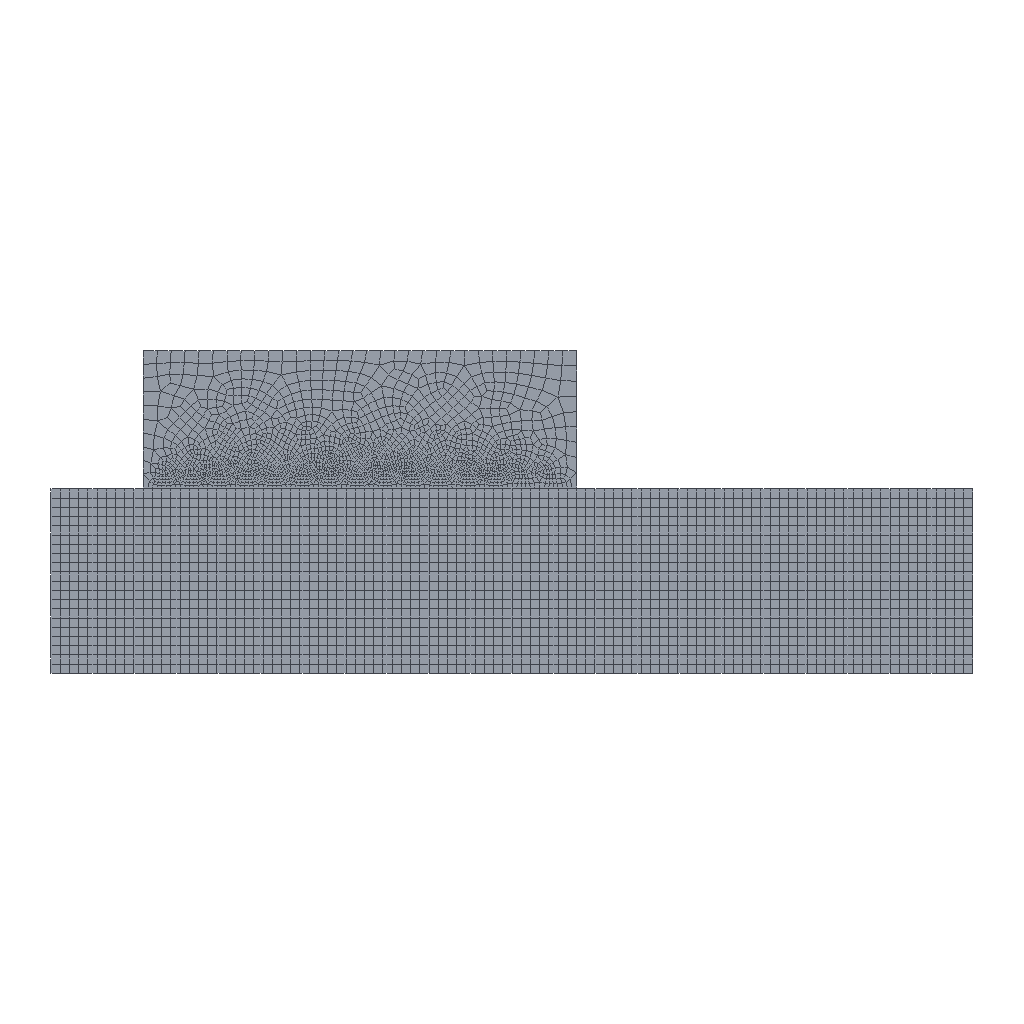Simulation study | abaqus
Set-up summary:
category,name,step,type,value,unit,region
solver,abaqus
solver,version,,,Abaqus/Explicit 2020
units,not stated in the deck,,not stated
analysis,deck,,transient,transient
load_step,Step-1,Step-1,transient,nlgeom=True
contact,interactions,,,general=1 pairs=0 ties=0
load_step,requested,,,1
mesh,nodes,,,4532
mesh,elements,,,4337
element_type,CPE4R,,plane,4243
element_type,COH2D4,,cohesive,94
load,load commands in deck,,count,2
bc,support commands in deck,,count,5
material,COH,,in results
material,FLUILD,,in results
material,MATERIAL-1,,in results
material,MATERIAL-3,,in results
check,setup vs results,,match,"per instance, exact: element labels, types and connectivity; labels of the nodes the elements use; coordinates of those nodes at SINGLE_PRECISION in 2 of 2 instance(s)"
Abaqus input file, long lists of numbers shortened:
*Heading
** Job name: Job-1 Model name: Model-1
** Generated by: Abaqus/CAE 2020
*Preprint, echo=NO, model=NO, history=NO, contact=NO
**
** PARTS
**
*Part, name=work-1
*Node
      1,           5.,          -3.
      2,    4.9,          -3.
** (2119 more lines like these left out)
*Element, type=CPE4R
   1,    1,    2,  103,  102
   2,    2,    3,  104,  103
** (1998 more lines like these left out)
*Nset, nset=Set-1, generate
    1,  2121,     1
*Elset, elset=Set-1, generate
    1,  2000,     1
** Section: steel
*Solid Section, elset=Set-1, material=Material-1
,
*End Part
**
*Part, name=work-2
*Node
      1,   -2.85,  -2.99
      2,  -2.7,  -2.99
** (2409 more lines like these left out)
*Element, type=CPE4R
 1,   1,  67, 412,  78
 2,  67,  68, 413, 412
** (2241 more lines like these left out)
*Element, type=COH2D4
205,  57, 231, 358,  62
206, 231, 232, 357, 358
** (92 more lines like these left out)
*Nset, nset=Set-1
   1,   2,   3,   4,   5,   6,   7,   8,   9,  10,  11,  12,  13,  14,  15,  16
  17,  18,  19,  20,  21,  22,  23,  24,  25,  26,  27,  28,  29,  30,  31,  32
** (20 more lines like these left out)
*Elset, elset=Set-1
   1,   2,   3,   4,   5,   6,   7,   8,   9,  10,  11,  12,  13,  14,  15,  16
  17,  18,  19,  20,  21,  22,  23,  24,  25,  26,  27,  28,  29,  30,  31,  32
** (12 more lines like these left out)
*Nset, nset=Set-2
    1,    2,    3,    4,    5,    6,    7,    8,    9,   10,   11,   12,   13,   14,   15,   16
   17,   18,   19,   20,   21,   22,   23,   24,   25,   26,   27,   28,   29,   30,   31,   32
** (134 more lines like these left out)
*Elset, elset=Set-2, generate
  308,  2337,     1
*Nset, nset=Set-3
   1,   2,   5,   6,   9,  10,  13,  14,  17,  18,  21,  22,  25,  26,  29,  30
  33,  34,  37,  38,  41,  42,  45,  46,  49,  50,  53,  54,  57,  58,  59,  60
** (10 more lines like these left out)
*Elset, elset=Set-3, generate
 205,  298,    1
*Nset, nset=Set-13
   1,   2,   5,   6,   9,  10,  13,  14,  17,  18,  21,  22,  25,  26,  29,  30
  33,  34,  37,  38,  41,  42,  45,  46,  49,  50,  53,  54,  57,  58,  59,  60
** (10 more lines like these left out)
*Elset, elset=Set-13, generate
 205,  298,    1
** Section: fluild
*Solid Section, elset=Set-1, material=fluild
,
** Section: coh
*Cohesive Section, elset=Set-13, controls=EC-1, material=coh, response=TRACTION SEPARATION
,
** Section: juxianyaan
*Solid Section, elset=Set-2, material=Material-3
,
*End Part
**
**
** ASSEMBLY
**
*Assembly, name=Assembly
**
*Instance, name=work-1-1, part=work-1
          1.,           0.,           0.
*End Instance
**
*Instance, name=work-2-1, part=work-2
*End Instance
**
*Nset, nset=Set-1, instance=work-2-1
  57,  60,  65,  66, 365, 366, 367, 368, 369, 370, 371, 372, 373, 374, 375, 376
 377, 378, 379, 380, 381, 382, 383, 384, 385, 386, 387, 388, 389, 390, 391, 392
** (2 more lines like these left out)
*Elset, elset=Set-1, instance=work-2-1
  319,  320,  321,  337,  338,  339,  341,  342,  343,  346,  347,  348,  349,  350,  351,  352
  353,  363,  372,  380,  392,  400,  410,  418,  430,  439,  440,  457,  458,  470,  471,  473
** (1 more lines like these left out)
*Nset, nset=Set-2, instance=work-1-1
    1,  101,  102,  202,  203,  303,  304,  404,  405,  505,  506,  606,  607,  707,  708,  808
  809,  909,  910, 1010, 1011, 1111, 1112, 1212, 1213, 1313, 1314, 1414, 1415, 1515, 1516, 1616
** (7 more lines like these left out)
*Elset, elset=Set-2, instance=work-1-1
    1,  100,  101,  200,  201,  300,  301,  400,  401,  500,  501,  600,  601,  700,  701,  800
  801,  900,  901, 1000, 1001, 1100, 1101, 1200, 1201, 1300, 1301, 1400, 1401, 1500, 1501, 1600
** (7 more lines like these left out)
*Elset, elset=_Surf-1_S4, internal, instance=work-2-1
 319, 320, 337, 351, 353, 372, 400, 418, 439, 457, 470
*Elset, elset=_Surf-1_S2, internal, instance=work-2-1
 321, 341, 342, 346, 348, 349, 352, 363, 380, 392, 410, 430, 440, 458, 603, 604
 605, 606, 607
*Elset, elset=_Surf-1_S3, internal, instance=work-2-1
 480,
*Surface, type=ELEMENT, name=Surf-1
_Surf-1_S4, S4
_Surf-1_S2, S2
_Surf-1_S3, S3
*End Assembly
**
** ELEMENT CONTROLS
**
*Section Controls, name=EC-1, ELEMENT DELETION=YES
1., 1., 1.
*Amplitude, name=Amp-1
             0.,              0.,            0.01,              1.
**
** MATERIALS
**
*Material, name=Material-1
*Density
 7.8e-09,
*Elastic
210000., 0.3
*Material, name=Material-3
*Density
 1.4e-09,
*Elastic
500., 0.34
*Material, name=coh
*Damage Initiation, criterion=MAXS
 0.11, 0.11, 0.11
*Damage Evolution, type=DISPLACEMENT
 1e-15,
*Density
 1.1e-09,
*Elastic, type=TRACTION
400.,400.,400.
*Material, name=fluild
*Density
 9e-10,
*Elastic
1., 0.4
**
** INTERACTION PROPERTIES
**
*Surface Interaction, name=IntProp-1
*Friction
 0.15,
*Surface Behavior, pressure-overclosure=HARD
**
** INTERACTIONS
**
** Interaction: Int-2
*Contact, op=NEW
*Contact Inclusions, ALL EXTERIOR
*Contact Property Assignment
 ,  , IntProp-1
** ----------------------------------------------------------------
**
** STEP: Step-1
**
*Step, name=Step-1, nlgeom=YES
*Dynamic, Explicit
, 0.01
*Bulk Viscosity
0.06, 1.2
**
** BOUNDARY CONDITIONS
**
** Name: BC-1 Type: 位移/转角
*Boundary
Set-1, 1, 1
Set-1, 6, 6
** Name: [REDACTED] : Displacement/rotation angle
*Boundary, amplitude=Amp-1
Set-2, 1, 1, -5.
Set-2, 2, 2
Set-2, 6, 6
**
** LOADS
**
** Name: Load-1   Type: Pressure
*Dsload
Surf-1, P, 5.
**
** OUTPUT REQUESTS
**
*Restart, write, number interval=1, time marks=NO
**
** FIELD OUTPUT: F-Output-1
**
*Output, field, number interval=50
*Node Output
CF, RF, RM, RT, U, V
*Element Output, directions=YES
E, LE, MISES, MISESMAX, PE, PEEQ, S, SDEG, SF, STATUS
*Contact Output
CDISP, CSTRESS
**
** HISTORY OUTPUT: H-Output-1
**
*Output, history, variable=PRESELECT
*End Step
Results summary:
result,step,Step-1,completed,increments=742256 time=0.01/0.01
result,analysis,,,transient
result,last_loadstep,,,1
result,analysis steps,,count,1
result,primary field,,,U
result,reaction total,,FX,-32.5,model units
result,reaction total,,FY,19.841,model units
result,reaction total,,FZ,0.0,model units